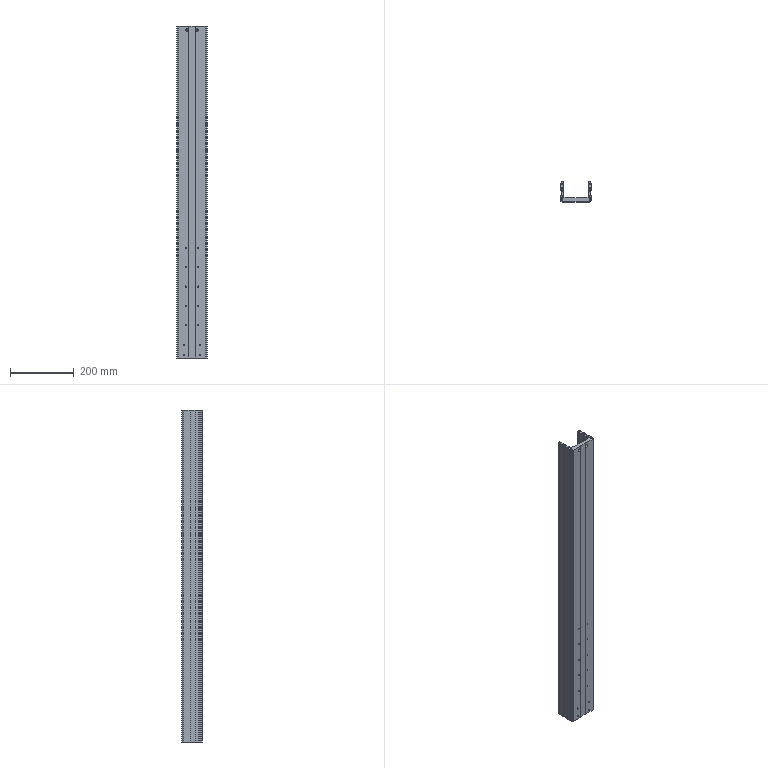Part | NX | 1 solid | 134 faces | box 95 x 64 x 1045 mm | volume 1787875 mm3 | plane 84 | cylinder 50 | commonest cylinder face diameters 1 x18 3.3 x10 2 x6 10 x6 3 x4 4.2 x4